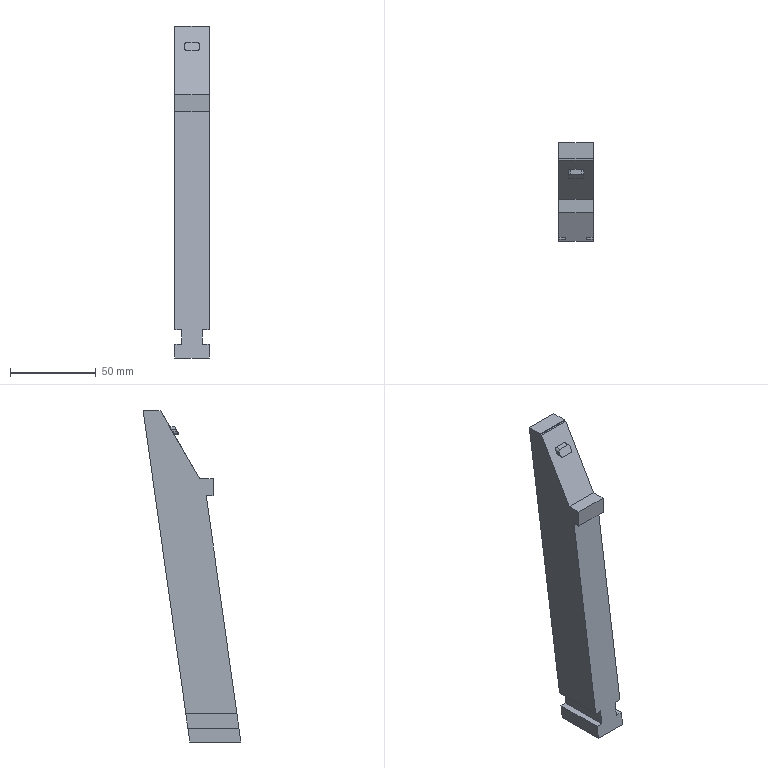Part | NX | features 模具.stp<1>[4] 2 | 1 solid | 29 faces | box 20 x 56.958 x 193.5 mm | volume 105226 mm3 | plane 25 | spline 4
STEP:
#1=CARTESIAN_POINT('',(-63.5,-228.097,-137.));
#2=VERTEX_POINT('',#1);
#3=CARTESIAN_POINT('',(-67.5,-228.097,-137.));
#4=VERTEX_POINT('',#3);
#5=CARTESIAN_POINT('',(38.,-228.097,-137.));
#6=DIRECTION('',(-1.,0.,0.));
#7=VECTOR('',#6,1000.);
#8=LINE('',#5,#7);
#9=EDGE_CURVE('',#2,#4,#8,.T.);
#10=ORIENTED_EDGE('',*,*,#9,.T.);
#11=CARTESIAN_POINT('',(-67.5,-198.334,-137.));
#12=VERTEX_POINT('',#11);
#13=CARTESIAN_POINT('',(-67.5,-264.,-137.));
#14=DIRECTION('',(0.,1.,0.));
#15=VECTOR('',#14,1000.);
#16=LINE('',#13,#15);
#17=EDGE_CURVE('',#4,#12,#16,.T.);
#18=ORIENTED_EDGE('',*,*,#17,.T.);
#19=CARTESIAN_POINT('',(-63.5,-198.334,-137.));
#20=VERTEX_POINT('',#19);
#21=CARTESIAN_POINT('',(38.,-198.334,-137.));
#22=DIRECTION('',(1.,0.,0.));
#23=VECTOR('',#22,1000.);
#24=LINE('',#21,#23);
#25=EDGE_CURVE('',#12,#20,#24,.T.);
#26=ORIENTED_EDGE('',*,*,#25,.T.);
#27=CARTESIAN_POINT('',(-63.5,-264.,-137.));
#28=DIRECTION('',(0.,-1.,0.));
#29=VECTOR('',#28,1000.);
#30=LINE('',#27,#29);
#31=EDGE_CURVE('',#20,#2,#30,.T.);
#32=ORIENTED_EDGE('',*,*,#31,.T.);
#33=EDGE_LOOP('',(#10,#18,#26,#32));
#34=FACE_BOUND('',#33,.T.);
#35=CARTESIAN_POINT('',(-63.5,-264.,-137.));
#36=DIRECTION('',(0.,0.,-1.));
#37=DIRECTION('',(-1.,0.,0.));
#38=AXIS2_PLACEMENT_3D('',#35,#36,#37);
#39=PLANE('',#38);
#40=ADVANCED_FACE('',(#34),#39,.T.);
#41=CARTESIAN_POINT('',(-63.5,-229.292,-145.5));
#42=VERTEX_POINT('',#41);
#43=CARTESIAN_POINT('',(-63.5,-210.249,-10.));
#44=DIRECTION('',(0.,0.1392,0.9903));
#45=VECTOR('',#44,1000.);
#46=LINE('',#43,#45);
#47=EDGE_CURVE('',#42,#2,#46,.T.);
#48=ORIENTED_EDGE('',*,*,#47,.T.);
#49=ORIENTED_EDGE('',*,*,#31,.F.);
#50=CARTESIAN_POINT('',(-63.5,-199.528,-145.5));
#51=VERTEX_POINT('',#50);
#52=CARTESIAN_POINT('',(-63.5,-193.248,-100.81));
#53=DIRECTION('',(0.,-0.1392,-0.9903));
#54=VECTOR('',#53,1000.);
#55=LINE('',#52,#54);
#56=EDGE_CURVE('',#20,#51,#55,.T.);
#57=ORIENTED_EDGE('',*,*,#56,.T.);
#58=CARTESIAN_POINT('',(-63.5,-264.,-145.5));
#59=DIRECTION('',(0.,-1.,0.));
#60=VECTOR('',#59,1000.);
#61=LINE('',#58,#60);
#62=EDGE_CURVE('',#51,#42,#61,.T.);
#63=ORIENTED_EDGE('',*,*,#62,.T.);
#64=EDGE_LOOP('',(#48,#49,#57,#63));
#65=FACE_BOUND('',#64,.T.);
#66=CARTESIAN_POINT('',(-63.5,-264.,-145.5));
#67=DIRECTION('',(-1.,0.,0.));
#68=DIRECTION('',(0.,0.,1.));
#69=AXIS2_PLACEMENT_3D('',#66,#67,#68);
#70=PLANE('',#69);
#71=ADVANCED_FACE('',(#65),#70,.T.);
#72=CARTESIAN_POINT('',(-67.5,-229.292,-145.5));
#73=VERTEX_POINT('',#72);
#74=CARTESIAN_POINT('',(38.,-229.292,-145.5));
#75=DIRECTION('',(1.,0.,0.));
#76=VECTOR('',#75,1000.);
#77=LINE('',#74,#76);
#78=EDGE_CURVE('',#73,#42,#77,.T.);
#79=ORIENTED_EDGE('',*,*,#78,.T.);
#80=ORIENTED_EDGE('',*,*,#62,.F.);
#81=CARTESIAN_POINT('',(-67.5,-199.528,-145.5));
#82=VERTEX_POINT('',#81);
#83=CARTESIAN_POINT('',(38.,-199.528,-145.5));
#84=DIRECTION('',(-1.,0.,0.));
#85=VECTOR('',#84,1000.);
#86=LINE('',#83,#85);
#87=EDGE_CURVE('',#51,#82,#86,.T.);
#88=ORIENTED_EDGE('',*,*,#87,.T.);
#89=CARTESIAN_POINT('',(-67.5,-264.,-145.5));
#90=DIRECTION('',(0.,1.,0.));
#91=VECTOR('',#90,1000.);
#92=LINE('',#89,#91);
#93=EDGE_CURVE('',#73,#82,#92,.T.);
#94=ORIENTED_EDGE('',*,*,#93,.F.);
#95=EDGE_LOOP('',(#79,#80,#88,#94));
#96=FACE_BOUND('',#95,.T.);
#97=CARTESIAN_POINT('',(-67.5,-264.,-145.5));
#98=DIRECTION('',(0.,0.,1.));
#99=DIRECTION('',(1.,0.,0.));
#100=AXIS2_PLACEMENT_3D('',#97,#98,#99);
#101=PLANE('',#100);
#102=ADVANCED_FACE('',(#96),#101,.T.);
#103=CARTESIAN_POINT('',(-47.5,-228.097,-137.));
#104=VERTEX_POINT('',#103);
#105=CARTESIAN_POINT('',(-51.5,-228.097,-137.));
#106=VERTEX_POINT('',#105);
#107=CARTESIAN_POINT('',(38.,-228.097,-137.));
#108=DIRECTION('',(-1.,0.,0.));
#109=VECTOR('',#108,1000.);
#110=LINE('',#107,#109);
#111=EDGE_CURVE('',#104,#106,#110,.T.);
#112=ORIENTED_EDGE('',*,*,#111,.T.);
#113=CARTESIAN_POINT('',(-51.5,-198.334,-137.));
#114=VERTEX_POINT('',#113);
#115=CARTESIAN_POINT('',(-51.5,-264.,-137.));
#116=DIRECTION('',(0.,1.,0.));
#117=VECTOR('',#116,1000.);
#118=LINE('',#115,#117);
#119=EDGE_CURVE('',#106,#114,#118,.T.);
#120=ORIENTED_EDGE('',*,*,#119,.T.);
#121=CARTESIAN_POINT('',(-47.5,-198.334,-137.));
#122=VERTEX_POINT('',#121);
#123=CARTESIAN_POINT('',(38.,-198.334,-137.));
#124=DIRECTION('',(1.,0.,0.));
#125=VECTOR('',#124,1000.);
#126=LINE('',#123,#125);
#127=EDGE_CURVE('',#114,#122,#126,.T.);
#128=ORIENTED_EDGE('',*,*,#127,.T.);
#129=CARTESIAN_POINT('',(-47.5,-264.,-137.));
#130=DIRECTION('',(0.,-1.,0.));
#131=VECTOR('',#130,1000.);
#132=LINE('',#129,#131);
#133=EDGE_CURVE('',#122,#104,#132,.T.);
#134=ORIENTED_EDGE('',*,*,#133,.T.);
#135=EDGE_LOOP('',(#112,#120,#128,#134));
#136=FACE_BOUND('',#135,.T.);
#137=CARTESIAN_POINT('',(-51.5,-264.,-137.));
#138=DIRECTION('',(0.,0.,-1.));
#139=DIRECTION('',(0.,-1.,0.));
#140=AXIS2_PLACEMENT_3D('',#137,#138,#139);
#141=PLANE('',#140);
#142=ADVANCED_FACE('',(#136),#141,.T.);
#143=CARTESIAN_POINT('',(-51.5,-229.292,-145.5));
#144=VERTEX_POINT('',#143);
#145=CARTESIAN_POINT('',(-51.5,-210.249,-10.));
#146=DIRECTION('',(0.,-0.1392,-0.9903));
#147=VECTOR('',#146,1000.);
#148=LINE('',#145,#147);
#149=EDGE_CURVE('',#106,#144,#148,.T.);
#150=ORIENTED_EDGE('',*,*,#149,.T.);
#151=CARTESIAN_POINT('',(-51.5,-199.528,-145.5));
#152=VERTEX_POINT('',#151);
#153=CARTESIAN_POINT('',(-51.5,-264.,-145.5));
#154=DIRECTION('',(0.,1.,0.));
#155=VECTOR('',#154,1000.);
#156=LINE('',#153,#155);
#157=EDGE_CURVE('',#144,#152,#156,.T.);
#158=ORIENTED_EDGE('',*,*,#157,.T.);
#159=CARTESIAN_POINT('',(-51.5,-193.248,-100.81));
#160=DIRECTION('',(0.,0.1392,0.9903));
#161=VECTOR('',#160,1000.);
#162=LINE('',#159,#161);
#163=EDGE_CURVE('',#152,#114,#162,.T.);
#164=ORIENTED_EDGE('',*,*,#163,.T.);
#165=ORIENTED_EDGE('',*,*,#119,.F.);
#166=EDGE_LOOP('',(#150,#158,#164,#165));
#167=FACE_BOUND('',#166,.T.);
#168=CARTESIAN_POINT('',(-51.5,-264.,-145.5));
#169=DIRECTION('',(1.,0.,0.));
#170=DIRECTION('',(0.,0.,-1.));
#171=AXIS2_PLACEMENT_3D('',#168,#169,#170);
#172=PLANE('',#171);
#173=ADVANCED_FACE('',(#167),#172,.T.);
#174=CARTESIAN_POINT('',(-47.5,-229.292,-145.5));
#175=VERTEX_POINT('',#174);
#176=CARTESIAN_POINT('',(38.,-229.292,-145.5));
#177=DIRECTION('',(1.,0.,0.));
#178=VECTOR('',#177,1000.);
#179=LINE('',#176,#178);
#180=EDGE_CURVE('',#144,#175,#179,.T.);
#181=ORIENTED_EDGE('',*,*,#180,.T.);
#182=CARTESIAN_POINT('',(-47.5,-199.528,-145.5));
#183=VERTEX_POINT('',#182);
#184=CARTESIAN_POINT('',(-47.5,-264.,-145.5));
#185=DIRECTION('',(0.,-1.,0.));
#186=VECTOR('',#185,1000.);
#187=LINE('',#184,#186);
#188=EDGE_CURVE('',#183,#175,#187,.T.);
#189=ORIENTED_EDGE('',*,*,#188,.F.);
#190=CARTESIAN_POINT('',(38.,-199.528,-145.5));
#191=DIRECTION('',(-1.,0.,0.));
#192=VECTOR('',#191,1000.);
#193=LINE('',#190,#192);
#194=EDGE_CURVE('',#183,#152,#193,.T.);
#195=ORIENTED_EDGE('',*,*,#194,.T.);
#196=ORIENTED_EDGE('',*,*,#157,.F.);
#197=EDGE_LOOP('',(#181,#189,#195,#196));
#198=FACE_BOUND('',#197,.T.);
#199=CARTESIAN_POINT('',(-47.5,-264.,-145.5));
#200=DIRECTION('',(0.,0.,1.));
#201=DIRECTION('',(1.,0.,0.));
#202=AXIS2_PLACEMENT_3D('',#199,#200,#201);
#203=PLANE('',#202);
#204=ADVANCED_FACE('',(#198),#203,.T.);
#205=CARTESIAN_POINT('',(-60.5,-191.803,30.217));
#206=VERTEX_POINT('',#205);
#207=CARTESIAN_POINT('',(-54.5,-191.803,30.217));
#208=VERTEX_POINT('',#207);
#209=CARTESIAN_POINT('',(0.,-191.803,30.217));
#210=DIRECTION('',(1.,0.,0.));
#211=VECTOR('',#210,1000.);
#212=LINE('',#209,#211);
#213=EDGE_CURVE('',#206,#208,#212,.T.);
#214=ORIENTED_EDGE('',*,*,#213,.F.);
#215=CARTESIAN_POINT('',(-62.,-192.553,28.917));
#216=VERTEX_POINT('',#215);
#217=CARTESIAN_POINT('',(-62.,-192.553,28.917));
#218=CARTESIAN_POINT('',(-62.,-192.455,29.088));
#219=CARTESIAN_POINT('',(-61.961,-192.357,29.258));
#220=CARTESIAN_POINT('',(-61.811,-192.175,29.572));
#221=CARTESIAN_POINT('',(-61.7,-192.092,29.716));
#222=CARTESIAN_POINT('',(-61.422,-191.953,29.956));
#223=CARTESIAN_POINT('',(-61.255,-191.898,30.053));
#224=CARTESIAN_POINT('',(-60.893,-191.823,30.183));
#225=CARTESIAN_POINT('',(-60.696,-191.803,30.217));
#226=CARTESIAN_POINT('',(-60.5,-191.803,30.217));
#227=B_SPLINE_CURVE_WITH_KNOTS('',3,(#217,#218,#219,#220,#221,#222,#223,#224,#225,#226),.UNSPECIFIED.,.F.,.F.,(4,2,2,2,4),(0.,0.25,0.5,0.75,1.),.UNSPECIFIED.);
#228=EDGE_CURVE('',#216,#206,#227,.T.);
#229=ORIENTED_EDGE('',*,*,#228,.F.);
#230=CARTESIAN_POINT('',(-62.,-193.553,27.185));
#231=VERTEX_POINT('',#230);
#232=CARTESIAN_POINT('',(-62.,-197.846,19.75));
#233=DIRECTION('',(0.,-0.5,-0.866));
#234=VECTOR('',#233,1000.);
#235=LINE('',#232,#234);
#236=EDGE_CURVE('',#216,#231,#235,.T.);
#237=ORIENTED_EDGE('',*,*,#236,.T.);
#238=CARTESIAN_POINT('',(-60.5,-194.303,25.886));
#239=VERTEX_POINT('',#238);
#240=CARTESIAN_POINT('',(-60.5,-194.303,25.886));
#241=CARTESIAN_POINT('',(-60.304,-194.303,25.886));
#242=CARTESIAN_POINT('',(-60.107,-194.284,25.92));
#243=CARTESIAN_POINT('',(-59.745,-194.209,26.05));
#244=CARTESIAN_POINT('',(-59.578,-194.153,26.147));
#245=CARTESIAN_POINT('',(-59.3,-194.014,26.387));
#246=CARTESIAN_POINT('',(-59.189,-193.931,26.531));
#247=CARTESIAN_POINT('',(-59.039,-193.749,26.845));
#248=CARTESIAN_POINT('',(-59.,-193.651,27.015));
#249=CARTESIAN_POINT('',(-59.,-193.455,27.355));
#250=CARTESIAN_POINT('',(-59.039,-193.357,27.525));
#251=CARTESIAN_POINT('',(-59.189,-193.175,27.84));
#252=CARTESIAN_POINT('',(-59.3,-193.092,27.984));
#253=CARTESIAN_POINT('',(-59.578,-192.953,28.224));
#254=CARTESIAN_POINT('',(-59.745,-192.898,28.321));
#255=CARTESIAN_POINT('',(-60.107,-192.823,28.451));
#256=CARTESIAN_POINT('',(-60.304,-192.803,28.484));
#257=CARTESIAN_POINT('',(-60.696,-192.803,28.484));
#258=CARTESIAN_POINT('',(-60.893,-192.823,28.451));
#259=CARTESIAN_POINT('',(-61.255,-192.898,28.321));
#260=CARTESIAN_POINT('',(-61.422,-192.953,28.224));
#261=CARTESIAN_POINT('',(-61.7,-193.092,27.984));
#262=CARTESIAN_POINT('',(-61.811,-193.175,27.84));
#263=CARTESIAN_POINT('',(-61.961,-193.357,27.525));
#264=CARTESIAN_POINT('',(-62.,-193.455,27.355));
#265=CARTESIAN_POINT('',(-62.,-193.651,27.015));
#266=CARTESIAN_POINT('',(-61.961,-193.749,26.845));
#267=CARTESIAN_POINT('',(-61.811,-193.931,26.531));
#268=CARTESIAN_POINT('',(-61.7,-194.014,26.387));
#269=CARTESIAN_POINT('',(-61.422,-194.153,26.147));
#270=CARTESIAN_POINT('',(-61.255,-194.209,26.05));
#271=CARTESIAN_POINT('',(-60.893,-194.284,25.92));
#272=CARTESIAN_POINT('',(-60.696,-194.303,25.886));
#273=CARTESIAN_POINT('',(-60.5,-194.303,25.886));
#274=B_SPLINE_CURVE_WITH_KNOTS('',3,(#240,#241,#242,#243,#244,#245,#246,#247,#248,#249,#250,#251,#252,#253,#254,#255,#256,#257,#258,#259,#260,#261,#262,#263,#264,#265,#266,#267,#268,#269,#270,#271,#272,#273),.UNSPECIFIED.,.T.,.F.,(1,3,2,2,2,2,2,2,2,2,2,2,2,2,2,2,2,3,1),(-0.0625,0.,0.0625,0.125,0.1875,0.25,0.3125,0.375,0.4375,0.5,0.5625,0.625,0.6875,0.75,0.8125,0.875,0.9375,1.,1.062),.UNSPECIFIED.);
#275=EDGE_CURVE('',#231,#239,#274,.T.);
#276=ORIENTED_EDGE('',*,*,#275,.T.);
#277=CARTESIAN_POINT('',(-54.5,-194.303,25.886));
#278=VERTEX_POINT('',#277);
#279=CARTESIAN_POINT('',(0.,-194.303,25.886));
#280=DIRECTION('',(1.,0.,0.));
#281=VECTOR('',#280,1000.);
#282=LINE('',#279,#281);
#283=EDGE_CURVE('',#239,#278,#282,.T.);
#284=ORIENTED_EDGE('',*,*,#283,.T.);
#285=CARTESIAN_POINT('',(-53.,-193.553,27.185));
#286=VERTEX_POINT('',#285);
#287=CARTESIAN_POINT('',(-54.5,-194.303,25.886));
#288=CARTESIAN_POINT('',(-54.696,-194.303,25.886));
#289=CARTESIAN_POINT('',(-54.893,-194.284,25.92));
#290=CARTESIAN_POINT('',(-55.255,-194.209,26.05));
#291=CARTESIAN_POINT('',(-55.422,-194.153,26.147));
#292=CARTESIAN_POINT('',(-55.7,-194.014,26.387));
#293=CARTESIAN_POINT('',(-55.811,-193.931,26.531));
#294=CARTESIAN_POINT('',(-55.961,-193.749,26.845));
#295=CARTESIAN_POINT('',(-56.,-193.651,27.015));
#296=CARTESIAN_POINT('',(-56.,-193.455,27.355));
#297=CARTESIAN_POINT('',(-55.961,-193.357,27.525));
#298=CARTESIAN_POINT('',(-55.811,-193.175,27.84));
#299=CARTESIAN_POINT('',(-55.7,-193.092,27.984));
#300=CARTESIAN_POINT('',(-55.422,-192.953,28.224));
#301=CARTESIAN_POINT('',(-55.255,-192.898,28.321));
#302=CARTESIAN_POINT('',(-54.893,-192.823,28.451));
#303=CARTESIAN_POINT('',(-54.696,-192.803,28.484));
#304=CARTESIAN_POINT('',(-54.304,-192.803,28.484));
#305=CARTESIAN_POINT('',(-54.107,-192.823,28.451));
#306=CARTESIAN_POINT('',(-53.745,-192.898,28.321));
#307=CARTESIAN_POINT('',(-53.578,-192.953,28.224));
#308=CARTESIAN_POINT('',(-53.3,-193.092,27.984));
#309=CARTESIAN_POINT('',(-53.189,-193.175,27.84));
#310=CARTESIAN_POINT('',(-53.039,-193.357,27.525));
#311=CARTESIAN_POINT('',(-53.,-193.455,27.355));
#312=CARTESIAN_POINT('',(-53.,-193.651,27.015));
#313=CARTESIAN_POINT('',(-53.039,-193.749,26.845));
#314=CARTESIAN_POINT('',(-53.189,-193.931,26.531));
#315=CARTESIAN_POINT('',(-53.3,-194.014,26.387));
#316=CARTESIAN_POINT('',(-53.578,-194.153,26.147));
#317=CARTESIAN_POINT('',(-53.745,-194.209,26.05));
#318=CARTESIAN_POINT('',(-54.107,-194.284,25.92));
#319=CARTESIAN_POINT('',(-54.304,-194.303,25.886));
#320=CARTESIAN_POINT('',(-54.5,-194.303,25.886));
#321=B_SPLINE_CURVE_WITH_KNOTS('',3,(#287,#288,#289,#290,#291,#292,#293,#294,#295,#296,#297,#298,#299,#300,#301,#302,#303,#304,#305,#306,#307,#308,#309,#310,#311,#312,#313,#314,#315,#316,#317,#318,#319,#320),.UNSPECIFIED.,.T.,.F.,(1,3,2,2,2,2,2,2,2,2,2,2,2,2,2,2,2,3,1),(-0.0625,0.,0.0625,0.125,0.1875,0.25,0.3125,0.375,0.4375,0.5,0.5625,0.625,0.6875,0.75,0.8125,0.875,0.9375,1.,1.062),.UNSPECIFIED.);
#322=EDGE_CURVE('',#286,#278,#321,.T.);
#323=ORIENTED_EDGE('',*,*,#322,.F.);
#324=CARTESIAN_POINT('',(-53.,-192.553,28.917));
#325=VERTEX_POINT('',#324);
#326=CARTESIAN_POINT('',(-53.,-197.846,19.75));
#327=DIRECTION('',(0.,-0.5,-0.866));
#328=VECTOR('',#327,1000.);
#329=LINE('',#326,#328);
#330=EDGE_CURVE('',#325,#286,#329,.T.);
#331=ORIENTED_EDGE('',*,*,#330,.F.);
#332=CARTESIAN_POINT('',(-54.5,-193.303,27.618));
#333=CARTESIAN_POINT('',(-54.696,-193.303,27.618));
#334=CARTESIAN_POINT('',(-54.893,-193.284,27.652));
#335=CARTESIAN_POINT('',(-55.255,-193.209,27.782));
#336=CARTESIAN_POINT('',(-55.422,-193.153,27.879));
#337=CARTESIAN_POINT('',(-55.7,-193.014,28.119));
#338=CARTESIAN_POINT('',(-55.811,-192.931,28.263));
#339=CARTESIAN_POINT('',(-55.961,-192.749,28.577));
#340=CARTESIAN_POINT('',(-56.,-192.651,28.747));
#341=CARTESIAN_POINT('',(-56.,-192.455,29.088));
#342=CARTESIAN_POINT('',(-55.961,-192.357,29.258));
#343=CARTESIAN_POINT('',(-55.811,-192.175,29.572));
#344=CARTESIAN_POINT('',(-55.7,-192.092,29.716));
#345=CARTESIAN_POINT('',(-55.422,-191.953,29.956));
#346=CARTESIAN_POINT('',(-55.255,-191.898,30.053));
#347=CARTESIAN_POINT('',(-54.893,-191.823,30.183));
#348=CARTESIAN_POINT('',(-54.696,-191.803,30.217));
#349=CARTESIAN_POINT('',(-54.304,-191.803,30.217));
#350=CARTESIAN_POINT('',(-54.107,-191.823,30.183));
#351=CARTESIAN_POINT('',(-53.745,-191.898,30.053));
#352=CARTESIAN_POINT('',(-53.578,-191.953,29.956));
#353=CARTESIAN_POINT('',(-53.3,-192.092,29.716));
#354=CARTESIAN_POINT('',(-53.189,-192.175,29.572));
#355=CARTESIAN_POINT('',(-53.039,-192.357,29.258));
#356=CARTESIAN_POINT('',(-53.,-192.455,29.088));
#357=CARTESIAN_POINT('',(-53.,-192.651,28.747));
#358=CARTESIAN_POINT('',(-53.039,-192.749,28.577));
#359=CARTESIAN_POINT('',(-53.189,-192.931,28.263));
#360=CARTESIAN_POINT('',(-53.3,-193.014,28.119));
#361=CARTESIAN_POINT('',(-53.578,-193.153,27.879));
#362=CARTESIAN_POINT('',(-53.745,-193.209,27.782));
#363=CARTESIAN_POINT('',(-54.107,-193.284,27.652));
#364=CARTESIAN_POINT('',(-54.304,-193.303,27.618));
#365=CARTESIAN_POINT('',(-54.5,-193.303,27.618));
#366=B_SPLINE_CURVE_WITH_KNOTS('',3,(#332,#333,#334,#335,#336,#337,#338,#339,#340,#341,#342,#343,#344,#345,#346,#347,#348,#349,#350,#351,#352,#353,#354,#355,#356,#357,#358,#359,#360,#361,#362,#363,#364,#365),.UNSPECIFIED.,.T.,.F.,(1,3,2,2,2,2,2,2,2,2,2,2,2,2,2,2,2,3,1),(-0.0625,0.,0.0625,0.125,0.1875,0.25,0.3125,0.375,0.4375,0.5,0.5625,0.625,0.6875,0.75,0.8125,0.875,0.9375,1.,1.062),.UNSPECIFIED.);
#367=EDGE_CURVE('',#208,#325,#366,.T.);
#368=ORIENTED_EDGE('',*,*,#367,.F.);
#369=EDGE_LOOP('',(#214,#229,#237,#276,#284,#323,#331,#368));
#370=FACE_BOUND('',#369,.T.);
#371=CARTESIAN_POINT('',(-337.196,-186.443,39.5));
#372=DIRECTION('',(0.,-0.866,0.5));
#373=DIRECTION('',(-1.,0.,0.));
#374=AXIS2_PLACEMENT_3D('',#371,#372,#373);
#375=PLANE('',#374);
#376=ADVANCED_FACE('',(#370),#375,.T.);
#377=CARTESIAN_POINT('',(-60.5,-188.916,30.217));
#378=VERTEX_POINT('',#377);
#379=CARTESIAN_POINT('',(-62.,-189.666,28.917));
#380=VERTEX_POINT('',#379);
#381=CARTESIAN_POINT('',(-60.5,-188.916,30.217));
#382=CARTESIAN_POINT('',(-60.696,-188.916,30.217));
#383=CARTESIAN_POINT('',(-60.893,-188.936,30.183));
#384=CARTESIAN_POINT('',(-61.255,-189.011,30.053));
#385=CARTESIAN_POINT('',(-61.422,-189.067,29.956));
#386=CARTESIAN_POINT('',(-61.7,-189.206,29.716));
#387=CARTESIAN_POINT('',(-61.811,-189.289,29.572));
#388=CARTESIAN_POINT('',(-61.961,-189.47,29.258));
#389=CARTESIAN_POINT('',(-62.,-189.568,29.088));
#390=CARTESIAN_POINT('',(-62.,-189.666,28.917));
#391=B_SPLINE_CURVE_WITH_KNOTS('',3,(#381,#382,#383,#384,#385,#386,#387,#388,#389,#390),.UNSPECIFIED.,.F.,.F.,(4,2,2,2,4),(0.,0.25,0.5,0.75,1.),.UNSPECIFIED.);
#392=EDGE_CURVE('',#378,#380,#391,.T.);
#393=ORIENTED_EDGE('',*,*,#392,.T.);
#394=CARTESIAN_POINT('',(-62.,-192.553,28.917));
#395=DIRECTION('',(0.,1.,0.));
#396=VECTOR('',#395,1000.);
#397=LINE('',#394,#396);
#398=EDGE_CURVE('',#216,#380,#397,.T.);
#399=ORIENTED_EDGE('',*,*,#398,.F.);
#400=ORIENTED_EDGE('',*,*,#228,.T.);
#401=CARTESIAN_POINT('',(-60.5,-191.803,30.217));
#402=DIRECTION('',(0.,1.,0.));
#403=VECTOR('',#402,1000.);
#404=LINE('',#401,#403);
#405=EDGE_CURVE('',#206,#378,#404,.T.);
#406=ORIENTED_EDGE('',*,*,#405,.T.);
#407=EDGE_LOOP('',(#393,#399,#400,#406));
#408=FACE_BOUND('',#407,.T.);
#409=CARTESIAN_POINT('',(-60.5,-191.803,30.217));
#410=CARTESIAN_POINT('',(-60.696,-191.803,30.217));
#411=CARTESIAN_POINT('',(-60.893,-191.823,30.183));
#412=CARTESIAN_POINT('',(-61.255,-191.898,30.053));
#413=CARTESIAN_POINT('',(-61.422,-191.953,29.956));
#414=CARTESIAN_POINT('',(-61.7,-192.092,29.716));
#415=CARTESIAN_POINT('',(-61.811,-192.175,29.572));
#416=CARTESIAN_POINT('',(-61.961,-192.357,29.258));
#417=CARTESIAN_POINT('',(-62.,-192.455,29.088));
#418=CARTESIAN_POINT('',(-62.,-192.553,28.917));
#419=CARTESIAN_POINT('',(-60.5,-188.916,30.217));
#420=CARTESIAN_POINT('',(-60.696,-188.916,30.217));
#421=CARTESIAN_POINT('',(-60.893,-188.936,30.183));
#422=CARTESIAN_POINT('',(-61.255,-189.011,30.053));
#423=CARTESIAN_POINT('',(-61.422,-189.067,29.956));
#424=CARTESIAN_POINT('',(-61.7,-189.206,29.716));
#425=CARTESIAN_POINT('',(-61.811,-189.289,29.572));
#426=CARTESIAN_POINT('',(-61.961,-189.47,29.258));
#427=CARTESIAN_POINT('',(-62.,-189.568,29.088));
#428=CARTESIAN_POINT('',(-62.,-189.666,28.917));
#429=B_SPLINE_SURFACE_WITH_KNOTS('',1,3,((#409,#410,#411,#412,#413,#414,#415,#416,#417,#418),(#419,#420,#421,#422,#423,#424,#425,#426,#427,#428)),.SURF_OF_LINEAR_EXTRUSION.,.F.,.F.,.F.,(2,2),(4,2,2,2,4),(0.1699,0.7147),(0.5,0.5625,0.625,0.6875,0.75),.UNSPECIFIED.);
#430=ADVANCED_FACE('',(#408),#429,.T.);
#431=ORIENTED_EDGE('',*,*,#398,.T.);
#432=CARTESIAN_POINT('',(-62.,-190.666,27.185));
#433=VERTEX_POINT('',#432);
#434=CARTESIAN_POINT('',(-62.,-182.835,40.75));
#435=DIRECTION('',(0.,0.5,0.866));
#436=VECTOR('',#435,1000.);
#437=LINE('',#434,#436);
#438=EDGE_CURVE('',#433,#380,#437,.T.);
#439=ORIENTED_EDGE('',*,*,#438,.F.);
#440=CARTESIAN_POINT('',(-62.,-193.553,27.185));
#441=DIRECTION('',(0.,1.,0.));
#442=VECTOR('',#441,1000.);
#443=LINE('',#440,#442);
#444=EDGE_CURVE('',#231,#433,#443,.T.);
#445=ORIENTED_EDGE('',*,*,#444,.F.);
#446=ORIENTED_EDGE('',*,*,#236,.F.);
#447=EDGE_LOOP('',(#431,#439,#445,#446));
#448=FACE_BOUND('',#447,.T.);
#449=CARTESIAN_POINT('',(-62.,-197.846,19.75));
#450=DIRECTION('',(1.,0.,0.));
#451=DIRECTION('',(0.,0.,-1.));
#452=AXIS2_PLACEMENT_3D('',#449,#450,#451);
#453=PLANE('',#452);
#454=ADVANCED_FACE('',(#448),#453,.F.);
#455=ORIENTED_EDGE('',*,*,#444,.T.);
#456=CARTESIAN_POINT('',(-60.5,-191.416,25.886));
#457=VERTEX_POINT('',#456);
#458=CARTESIAN_POINT('',(-60.5,-191.416,25.886));
#459=CARTESIAN_POINT('',(-60.696,-191.416,25.886));
#460=CARTESIAN_POINT('',(-60.893,-191.397,25.92));
#461=CARTESIAN_POINT('',(-61.255,-191.322,26.05));
#462=CARTESIAN_POINT('',(-61.422,-191.266,26.147));
#463=CARTESIAN_POINT('',(-61.7,-191.127,26.387));
#464=CARTESIAN_POINT('',(-61.811,-191.044,26.531));
#465=CARTESIAN_POINT('',(-61.961,-190.863,26.845));
#466=CARTESIAN_POINT('',(-62.,-190.765,27.015));
#467=CARTESIAN_POINT('',(-62.,-190.666,27.185));
#468=B_SPLINE_CURVE_WITH_KNOTS('',3,(#458,#459,#460,#461,#462,#463,#464,#465,#466,#467),.UNSPECIFIED.,.F.,.F.,(4,2,2,2,4),(0.,0.25,0.5,0.75,1.),.UNSPECIFIED.);
#469=EDGE_CURVE('',#457,#433,#468,.T.);
#470=ORIENTED_EDGE('',*,*,#469,.F.);
#471=CARTESIAN_POINT('',(-60.5,-194.303,25.886));
#472=DIRECTION('',(0.,1.,0.));
#473=VECTOR('',#472,1000.);
#474=LINE('',#471,#473);
#475=EDGE_CURVE('',#239,#457,#474,.T.);
#476=ORIENTED_EDGE('',*,*,#475,.F.);
#477=ORIENTED_EDGE('',*,*,#275,.F.);
#478=EDGE_LOOP('',(#455,#470,#476,#477));
#479=FACE_BOUND('',#478,.T.);
#480=CARTESIAN_POINT('',(-62.,-193.553,27.185));
#481=CARTESIAN_POINT('',(-62.,-193.651,27.015));
#482=CARTESIAN_POINT('',(-61.961,-193.749,26.845));
#483=CARTESIAN_POINT('',(-61.811,-193.931,26.531));
#484=CARTESIAN_POINT('',(-61.7,-194.014,26.387));
#485=CARTESIAN_POINT('',(-61.422,-194.153,26.147));
#486=CARTESIAN_POINT('',(-61.255,-194.209,26.05));
#487=CARTESIAN_POINT('',(-60.893,-194.284,25.92));
#488=CARTESIAN_POINT('',(-60.696,-194.303,25.886));
#489=CARTESIAN_POINT('',(-60.5,-194.303,25.886));
#490=CARTESIAN_POINT('',(-62.,-190.666,27.185));
#491=CARTESIAN_POINT('',(-62.,-190.765,27.015));
#492=CARTESIAN_POINT('',(-61.961,-190.863,26.845));
#493=CARTESIAN_POINT('',(-61.811,-191.044,26.531));
#494=CARTESIAN_POINT('',(-61.7,-191.127,26.387));
#495=CARTESIAN_POINT('',(-61.422,-191.266,26.147));
#496=CARTESIAN_POINT('',(-61.255,-191.322,26.05));
#497=CARTESIAN_POINT('',(-60.893,-191.397,25.92));
#498=CARTESIAN_POINT('',(-60.696,-191.416,25.886));
#499=CARTESIAN_POINT('',(-60.5,-191.416,25.886));
#500=B_SPLINE_SURFACE_WITH_KNOTS('',1,3,((#480,#481,#482,#483,#484,#485,#486,#487,#488,#489),(#490,#491,#492,#493,#494,#495,#496,#497,#498,#499)),.SURF_OF_LINEAR_EXTRUSION.,.F.,.F.,.F.,(2,2),(4,2,2,2,4),(0.3397,0.8846),(0.75,0.8125,0.875,0.9375,1.),.UNSPECIFIED.);
#501=ADVANCED_FACE('',(#479),#500,.T.);
#502=ORIENTED_EDGE('',*,*,#475,.T.);
#503=CARTESIAN_POINT('',(-54.5,-191.416,25.886));
#504=VERTEX_POINT('',#503);
#505=CARTESIAN_POINT('',(-89.,-191.416,25.886));
#506=DIRECTION('',(-1.,0.,0.));
#507=VECTOR('',#506,1000.);
#508=LINE('',#505,#507);
#509=EDGE_CURVE('',#504,#457,#508,.T.);
#510=ORIENTED_EDGE('',*,*,#509,.F.);
#511=CARTESIAN_POINT('',(-54.5,-194.303,25.886));
#512=DIRECTION('',(0.,1.,0.));
#513=VECTOR('',#512,1000.);
#514=LINE('',#511,#513);
#515=EDGE_CURVE('',#278,#504,#514,.T.);
#516=ORIENTED_EDGE('',*,*,#515,.F.);
#517=ORIENTED_EDGE('',*,*,#283,.F.);
#518=EDGE_LOOP('',(#502,#510,#516,#517));
#519=FACE_BOUND('',#518,.T.);
#520=CARTESIAN_POINT('',(0.,-194.303,25.886));
#521=DIRECTION('',(0.,0.,1.));
#522=DIRECTION('',(1.,0.,0.));
#523=AXIS2_PLACEMENT_3D('',#520,#521,#522);
#524=PLANE('',#523);
#525=ADVANCED_FACE('',(#519),#524,.F.);
#526=CARTESIAN_POINT('',(-53.,-190.666,27.185));
#527=VERTEX_POINT('',#526);
#528=CARTESIAN_POINT('',(-54.5,-191.416,25.886));
#529=CARTESIAN_POINT('',(-54.304,-191.416,25.886));
#530=CARTESIAN_POINT('',(-54.107,-191.397,25.92));
#531=CARTESIAN_POINT('',(-53.745,-191.322,26.05));
#532=CARTESIAN_POINT('',(-53.578,-191.266,26.147));
#533=CARTESIAN_POINT('',(-53.3,-191.127,26.387));
#534=CARTESIAN_POINT('',(-53.189,-191.044,26.531));
#535=CARTESIAN_POINT('',(-53.039,-190.863,26.845));
#536=CARTESIAN_POINT('',(-53.,-190.765,27.015));
#537=CARTESIAN_POINT('',(-53.,-190.666,27.185));
#538=B_SPLINE_CURVE_WITH_KNOTS('',3,(#528,#529,#530,#531,#532,#533,#534,#535,#536,#537),.UNSPECIFIED.,.F.,.F.,(4,2,2,2,4),(0.,0.25,0.5,0.75,1.),.UNSPECIFIED.);
#539=EDGE_CURVE('',#504,#527,#538,.T.);
#540=ORIENTED_EDGE('',*,*,#539,.T.);
#541=CARTESIAN_POINT('',(-53.,-193.553,27.185));
#542=DIRECTION('',(0.,1.,0.));
#543=VECTOR('',#542,1000.);
#544=LINE('',#541,#543);
#545=EDGE_CURVE('',#286,#527,#544,.T.);
#546=ORIENTED_EDGE('',*,*,#545,.F.);
#547=ORIENTED_EDGE('',*,*,#322,.T.);
#548=ORIENTED_EDGE('',*,*,#515,.T.);
#549=EDGE_LOOP('',(#540,#546,#547,#548));
#550=FACE_BOUND('',#549,.T.);
#551=CARTESIAN_POINT('',(-54.5,-194.303,25.886));
#552=CARTESIAN_POINT('',(-54.304,-194.303,25.886));
#553=CARTESIAN_POINT('',(-54.107,-194.284,25.92));
#554=CARTESIAN_POINT('',(-53.745,-194.209,26.05));
#555=CARTESIAN_POINT('',(-53.578,-194.153,26.147));
#556=CARTESIAN_POINT('',(-53.3,-194.014,26.387));
#557=CARTESIAN_POINT('',(-53.189,-193.931,26.531));
#558=CARTESIAN_POINT('',(-53.039,-193.749,26.845));
#559=CARTESIAN_POINT('',(-53.,-193.651,27.015));
#560=CARTESIAN_POINT('',(-53.,-193.553,27.185));
#561=CARTESIAN_POINT('',(-54.5,-191.416,25.886));
#562=CARTESIAN_POINT('',(-54.304,-191.416,25.886));
#563=CARTESIAN_POINT('',(-54.107,-191.397,25.92));
#564=CARTESIAN_POINT('',(-53.745,-191.322,26.05));
#565=CARTESIAN_POINT('',(-53.578,-191.266,26.147));
#566=CARTESIAN_POINT('',(-53.3,-191.127,26.387));
#567=CARTESIAN_POINT('',(-53.189,-191.044,26.531));
#568=CARTESIAN_POINT('',(-53.039,-190.863,26.845));
#569=CARTESIAN_POINT('',(-53.,-190.765,27.015));
#570=CARTESIAN_POINT('',(-53.,-190.666,27.185));
#571=B_SPLINE_SURFACE_WITH_KNOTS('',1,3,((#551,#552,#553,#554,#555,#556,#557,#558,#559,#560),(#561,#562,#563,#564,#565,#566,#567,#568,#569,#570)),.SURF_OF_LINEAR_EXTRUSION.,.F.,.F.,.F.,(2,2),(4,2,2,2,4),(0.3397,0.8846),(0.,0.0625,0.125,0.1875,0.25),.UNSPECIFIED.);
#572=ADVANCED_FACE('',(#550),#571,.T.);
#573=CARTESIAN_POINT('',(-53.,-189.666,28.917));
#574=VERTEX_POINT('',#573);
#575=CARTESIAN_POINT('',(-53.,-182.835,40.75));
#576=DIRECTION('',(0.,0.5,0.866));
#577=VECTOR('',#576,1000.);
#578=LINE('',#575,#577);
#579=EDGE_CURVE('',#527,#574,#578,.T.);
#580=ORIENTED_EDGE('',*,*,#579,.T.);
#581=CARTESIAN_POINT('',(-53.,-192.553,28.917));
#582=DIRECTION('',(0.,1.,0.));
#583=VECTOR('',#582,1000.);
#584=LINE('',#581,#583);
#585=EDGE_CURVE('',#325,#574,#584,.T.);
#586=ORIENTED_EDGE('',*,*,#585,.F.);
#587=ORIENTED_EDGE('',*,*,#330,.T.);
#588=ORIENTED_EDGE('',*,*,#545,.T.);
#589=EDGE_LOOP('',(#580,#586,#587,#588));
#590=FACE_BOUND('',#589,.T.);
#591=CARTESIAN_POINT('',(-53.,-197.846,19.75));
#592=DIRECTION('',(-1.,0.,0.));
#593=DIRECTION('',(0.,1.,0.));
#594=AXIS2_PLACEMENT_3D('',#591,#592,#593);
#595=PLANE('',#594);
#596=ADVANCED_FACE('',(#590),#595,.F.);
#597=CARTESIAN_POINT('',(-54.5,-188.916,30.217));
#598=VERTEX_POINT('',#597);
#599=CARTESIAN_POINT('',(-53.,-189.666,28.917));
#600=CARTESIAN_POINT('',(-53.,-189.568,29.088));
#601=CARTESIAN_POINT('',(-53.039,-189.47,29.258));
#602=CARTESIAN_POINT('',(-53.189,-189.289,29.572));
#603=CARTESIAN_POINT('',(-53.3,-189.206,29.716));
#604=CARTESIAN_POINT('',(-53.578,-189.067,29.956));
#605=CARTESIAN_POINT('',(-53.745,-189.011,30.053));
#606=CARTESIAN_POINT('',(-54.107,-188.936,30.183));
#607=CARTESIAN_POINT('',(-54.304,-188.916,30.217));
#608=CARTESIAN_POINT('',(-54.5,-188.916,30.217));
#609=B_SPLINE_CURVE_WITH_KNOTS('',3,(#599,#600,#601,#602,#603,#604,#605,#606,#607,#608),.UNSPECIFIED.,.F.,.F.,(4,2,2,2,4),(0.,0.25,0.5,0.75,1.),.UNSPECIFIED.);
#610=EDGE_CURVE('',#574,#598,#609,.T.);
#611=ORIENTED_EDGE('',*,*,#610,.T.);
#612=CARTESIAN_POINT('',(-54.5,-191.803,30.217));
#613=DIRECTION('',(0.,1.,0.));
#614=VECTOR('',#613,1000.);
#615=LINE('',#612,#614);
#616=EDGE_CURVE('',#208,#598,#615,.T.);
#617=ORIENTED_EDGE('',*,*,#616,.F.);
#618=ORIENTED_EDGE('',*,*,#367,.T.);
#619=ORIENTED_EDGE('',*,*,#585,.T.);
#620=EDGE_LOOP('',(#611,#617,#618,#619));
#621=FACE_BOUND('',#620,.T.);
#622=CARTESIAN_POINT('',(-53.,-192.553,28.917));
#623=CARTESIAN_POINT('',(-53.,-192.455,29.088));
#624=CARTESIAN_POINT('',(-53.039,-192.357,29.258));
#625=CARTESIAN_POINT('',(-53.189,-192.175,29.572));
#626=CARTESIAN_POINT('',(-53.3,-192.092,29.716));
#627=CARTESIAN_POINT('',(-53.578,-191.953,29.956));
#628=CARTESIAN_POINT('',(-53.745,-191.898,30.053));
#629=CARTESIAN_POINT('',(-54.107,-191.823,30.183));
#630=CARTESIAN_POINT('',(-54.304,-191.803,30.217));
#631=CARTESIAN_POINT('',(-54.5,-191.803,30.217));
#632=CARTESIAN_POINT('',(-53.,-189.666,28.917));
#633=CARTESIAN_POINT('',(-53.,-189.568,29.088));
#634=CARTESIAN_POINT('',(-53.039,-189.47,29.258));
#635=CARTESIAN_POINT('',(-53.189,-189.289,29.572));
#636=CARTESIAN_POINT('',(-53.3,-189.206,29.716));
#637=CARTESIAN_POINT('',(-53.578,-189.067,29.956));
#638=CARTESIAN_POINT('',(-53.745,-189.011,30.053));
#639=CARTESIAN_POINT('',(-54.107,-188.936,30.183));
#640=CARTESIAN_POINT('',(-54.304,-188.916,30.217));
#641=CARTESIAN_POINT('',(-54.5,-188.916,30.217));
#642=B_SPLINE_SURFACE_WITH_KNOTS('',1,3,((#622,#623,#624,#625,#626,#627,#628,#629,#630,#631),(#632,#633,#634,#635,#636,#637,#638,#639,#640,#641)),.SURF_OF_LINEAR_EXTRUSION.,.F.,.F.,.F.,(2,2),(4,2,2,2,4),(0.1699,0.7147),(0.25,0.3125,0.375,0.4375,0.5),.UNSPECIFIED.);
#643=ADVANCED_FACE('',(#621),#642,.T.);
#644=CARTESIAN_POINT('',(-89.,-188.916,30.217));
#645=DIRECTION('',(-1.,0.,0.));
#646=VECTOR('',#645,1000.);
#647=LINE('',#644,#646);
#648=EDGE_CURVE('',#598,#378,#647,.T.);
#649=ORIENTED_EDGE('',*,*,#648,.T.);
#650=ORIENTED_EDGE('',*,*,#405,.F.);
#651=ORIENTED_EDGE('',*,*,#213,.T.);
#652=ORIENTED_EDGE('',*,*,#616,.T.);
#653=EDGE_LOOP('',(#649,#650,#651,#652));
#654=FACE_BOUND('',#653,.T.);
#655=CARTESIAN_POINT('',(0.,-191.803,30.217));
#656=DIRECTION('',(0.,0.,-1.));
#657=DIRECTION('',(-1.,0.,0.));
#658=AXIS2_PLACEMENT_3D('',#655,#656,#657);
#659=PLANE('',#658);
#660=ADVANCED_FACE('',(#654),#659,.F.);
#661=CARTESIAN_POINT('',(-47.5,-182.5,40.));
#662=VERTEX_POINT('',#661);
#663=CARTESIAN_POINT('',(-47.5,-173.458,40.));
#664=VERTEX_POINT('',#663);
#665=CARTESIAN_POINT('',(-47.5,-197.846,40.));
#666=DIRECTION('',(0.,1.,0.));
#667=VECTOR('',#666,1000.);
#668=LINE('',#665,#667);
#669=EDGE_CURVE('',#662,#664,#668,.T.);
#670=ORIENTED_EDGE('',*,*,#669,.T.);
#671=CARTESIAN_POINT('',(-67.5,-173.458,40.));
#672=VERTEX_POINT('',#671);
#673=CARTESIAN_POINT('',(38.,-173.458,40.));
#674=DIRECTION('',(1.,0.,0.));
#675=VECTOR('',#674,1000.);
#676=LINE('',#673,#675);
#677=EDGE_CURVE('',#672,#664,#676,.T.);
#678=ORIENTED_EDGE('',*,*,#677,.F.);
#679=CARTESIAN_POINT('',(-67.5,-182.5,40.));
#680=VERTEX_POINT('',#679);
#681=CARTESIAN_POINT('',(-67.5,-197.846,40.));
#682=DIRECTION('',(0.,1.,0.));
#683=VECTOR('',#682,1000.);
#684=LINE('',#681,#683);
#685=EDGE_CURVE('',#680,#672,#684,.T.);
#686=ORIENTED_EDGE('',*,*,#685,.F.);
#687=CARTESIAN_POINT('',(-89.,-182.5,40.));
#688=DIRECTION('',(1.,0.,0.));
#689=VECTOR('',#688,1000.);
#690=LINE('',#687,#689);
#691=EDGE_CURVE('',#680,#662,#690,.T.);
#692=ORIENTED_EDGE('',*,*,#691,.T.);
#693=EDGE_LOOP('',(#670,#678,#686,#692));
#694=FACE_BOUND('',#693,.T.);
#695=CARTESIAN_POINT('',(0.,0.,40.));
#696=DIRECTION('',(0.,0.,-1.));
#697=DIRECTION('',(0.,-1.,0.));
#698=AXIS2_PLACEMENT_3D('',#695,#696,#697);
#699=PLANE('',#698);
#700=ADVANCED_FACE('',(#694),#699,.F.);
#701=ORIENTED_EDGE('',*,*,#648,.F.);
#702=ORIENTED_EDGE('',*,*,#610,.F.);
#703=ORIENTED_EDGE('',*,*,#579,.F.);
#704=ORIENTED_EDGE('',*,*,#539,.F.);
#705=ORIENTED_EDGE('',*,*,#509,.T.);
#706=ORIENTED_EDGE('',*,*,#469,.T.);
#707=ORIENTED_EDGE('',*,*,#438,.T.);
#708=ORIENTED_EDGE('',*,*,#392,.F.);
#709=EDGE_LOOP('',(#701,#702,#703,#704,#705,#706,#707,#708));
#710=FACE_BOUND('',#709,.T.);
#711=CARTESIAN_POINT('',(-47.5,-206.362,0.));
#712=VERTEX_POINT('',#711);
#713=CARTESIAN_POINT('',(-47.5,-183.557,39.5));
#714=VERTEX_POINT('',#713);
#715=CARTESIAN_POINT('',(-47.5,-195.681,18.5));
#716=DIRECTION('',(0.,0.5,0.866));
#717=VECTOR('',#716,1000.);
#718=LINE('',#715,#717);
#719=EDGE_CURVE('',#712,#714,#718,.T.);
#720=ORIENTED_EDGE('',*,*,#719,.T.);
#721=CARTESIAN_POINT('',(-67.5,-183.557,39.5));
#722=VERTEX_POINT('',#721);
#723=CARTESIAN_POINT('',(0.,-183.557,39.5));
#724=DIRECTION('',(-1.,0.,0.));
#725=VECTOR('',#724,1000.);
#726=LINE('',#723,#725);
#727=EDGE_CURVE('',#714,#722,#726,.T.);
#728=ORIENTED_EDGE('',*,*,#727,.T.);
#729=CARTESIAN_POINT('',(-67.5,-206.362,0.));
#730=VERTEX_POINT('',#729);
#731=CARTESIAN_POINT('',(-67.5,-195.681,18.5));
#732=DIRECTION('',(0.,0.5,0.866));
#733=VECTOR('',#732,1000.);
#734=LINE('',#731,#733);
#735=EDGE_CURVE('',#730,#722,#734,.T.);
#736=ORIENTED_EDGE('',*,*,#735,.F.);
#737=CARTESIAN_POINT('',(-89.,-206.362,0.));
#738=DIRECTION('',(-1.,0.,0.));
#739=VECTOR('',#738,1000.);
#740=LINE('',#737,#739);
#741=EDGE_CURVE('',#712,#730,#740,.T.);
#742=ORIENTED_EDGE('',*,*,#741,.F.);
#743=EDGE_LOOP('',(#720,#728,#736,#742));
#744=FACE_BOUND('',#743,.T.);
#745=CARTESIAN_POINT('',(-89.,-182.835,40.75));
#746=DIRECTION('',(0.,-0.866,0.5));
#747=DIRECTION('',(-1.,0.,0.));
#748=AXIS2_PLACEMENT_3D('',#745,#746,#747);
#749=PLANE('',#748);
#750=ADVANCED_FACE('',(#710,#744),#749,.T.);
#751=CARTESIAN_POINT('',(-47.5,-182.5,39.5));
#752=VERTEX_POINT('',#751);
#753=CARTESIAN_POINT('',(-47.5,-197.846,39.5));
#754=DIRECTION('',(0.,1.,0.));
#755=VECTOR('',#754,1000.);
#756=LINE('',#753,#755);
#757=EDGE_CURVE('',#714,#752,#756,.T.);
#758=ORIENTED_EDGE('',*,*,#757,.T.);
#759=CARTESIAN_POINT('',(-67.5,-182.5,39.5));
#760=VERTEX_POINT('',#759);
#761=CARTESIAN_POINT('',(0.,-182.5,39.5));
#762=DIRECTION('',(1.,0.,0.));
#763=VECTOR('',#762,1000.);
#764=LINE('',#761,#763);
#765=EDGE_CURVE('',#760,#752,#764,.T.);
#766=ORIENTED_EDGE('',*,*,#765,.F.);
#767=CARTESIAN_POINT('',(-67.5,-197.846,39.5));
#768=DIRECTION('',(0.,1.,0.));
#769=VECTOR('',#768,1000.);
#770=LINE('',#767,#769);
#771=EDGE_CURVE('',#722,#760,#770,.T.);
#772=ORIENTED_EDGE('',*,*,#771,.F.);
#773=ORIENTED_EDGE('',*,*,#727,.F.);
#774=EDGE_LOOP('',(#758,#766,#772,#773));
#775=FACE_BOUND('',#774,.T.);
#776=CARTESIAN_POINT('',(0.,0.,39.5));
#777=DIRECTION('',(0.,0.,-1.));
#778=DIRECTION('',(0.,-1.,0.));
#779=AXIS2_PLACEMENT_3D('',#776,#777,#778);
#780=PLANE('',#779);
#781=ADVANCED_FACE('',(#775),#780,.F.);
#782=ORIENTED_EDGE('',*,*,#691,.F.);
#783=CARTESIAN_POINT('',(-67.5,-182.5,19.75));
#784=DIRECTION('',(0.,0.,-1.));
#785=VECTOR('',#784,1000.);
#786=LINE('',#783,#785);
#787=EDGE_CURVE('',#680,#760,#786,.T.);
#788=ORIENTED_EDGE('',*,*,#787,.T.);
#789=ORIENTED_EDGE('',*,*,#765,.T.);
#790=CARTESIAN_POINT('',(-47.5,-182.5,19.75));
#791=DIRECTION('',(0.,0.,-1.));
#792=VECTOR('',#791,1000.);
#793=LINE('',#790,#792);
#794=EDGE_CURVE('',#662,#752,#793,.T.);
#795=ORIENTED_EDGE('',*,*,#794,.F.);
#796=EDGE_LOOP('',(#782,#788,#789,#795));
#797=FACE_BOUND('',#796,.T.);
#798=CARTESIAN_POINT('',(0.,-182.5,40.));
#799=DIRECTION('',(0.,-1.,0.));
#800=DIRECTION('',(0.,0.,-1.));
#801=AXIS2_PLACEMENT_3D('',#798,#799,#800);
#802=PLANE('',#801);
#803=ADVANCED_FACE('',(#797),#802,.T.);
#804=CARTESIAN_POINT('',(-47.5,-214.249,0.));
#805=VERTEX_POINT('',#804);
#806=CARTESIAN_POINT('',(-47.5,-214.249,-10.));
#807=VERTEX_POINT('',#806);
#808=CARTESIAN_POINT('',(-47.5,-214.249,59.169));
#809=DIRECTION('',(0.,0.,-1.));
#810=VECTOR('',#809,1000.);
#811=LINE('',#808,#810);
#812=EDGE_CURVE('',#805,#807,#811,.T.);
#813=ORIENTED_EDGE('',*,*,#812,.F.);
#814=CARTESIAN_POINT('',(-67.5,-214.249,0.));
#815=VERTEX_POINT('',#814);
#816=CARTESIAN_POINT('',(38.,-214.249,0.));
#817=DIRECTION('',(-1.,0.,0.));
#818=VECTOR('',#817,1000.);
#819=LINE('',#816,#818);
#820=EDGE_CURVE('',#805,#815,#819,.T.);
#821=ORIENTED_EDGE('',*,*,#820,.T.);
#822=CARTESIAN_POINT('',(-67.5,-214.249,-10.));
#823=VERTEX_POINT('',#822);
#824=CARTESIAN_POINT('',(-67.5,-214.249,59.169));
#825=DIRECTION('',(0.,0.,-1.));
#826=VECTOR('',#825,1000.);
#827=LINE('',#824,#826);
#828=EDGE_CURVE('',#815,#823,#827,.T.);
#829=ORIENTED_EDGE('',*,*,#828,.T.);
#830=CARTESIAN_POINT('',(38.,-214.249,-10.));
#831=DIRECTION('',(-1.,0.,0.));
#832=VECTOR('',#831,1000.);
#833=LINE('',#830,#832);
#834=EDGE_CURVE('',#807,#823,#833,.T.);
#835=ORIENTED_EDGE('',*,*,#834,.F.);
#836=EDGE_LOOP('',(#813,#821,#829,#835));
#837=FACE_BOUND('',#836,.T.);
#838=CARTESIAN_POINT('',(38.,-214.249,59.169));
#839=DIRECTION('',(0.,1.,0.));
#840=DIRECTION('',(1.,0.,0.));
#841=AXIS2_PLACEMENT_3D('',#838,#839,#840);
#842=PLANE('',#841);
#843=ADVANCED_FACE('',(#837),#842,.F.);
#844=ORIENTED_EDGE('',*,*,#133,.F.);
#845=CARTESIAN_POINT('',(-47.5,-193.248,-100.81));
#846=DIRECTION('',(0.,0.1392,0.9903));
#847=VECTOR('',#846,1000.);
#848=LINE('',#845,#847);
#849=EDGE_CURVE('',#122,#664,#848,.T.);
#850=ORIENTED_EDGE('',*,*,#849,.T.);
#851=ORIENTED_EDGE('',*,*,#669,.F.);
#852=ORIENTED_EDGE('',*,*,#794,.T.);
#853=ORIENTED_EDGE('',*,*,#757,.F.);
#854=ORIENTED_EDGE('',*,*,#719,.F.);
#855=CARTESIAN_POINT('',(-47.5,-144.,0.));
#856=DIRECTION('',(0.,-1.,0.));
#857=VECTOR('',#856,1000.);
#858=LINE('',#855,#857);
#859=EDGE_CURVE('',#712,#805,#858,.T.);
#860=ORIENTED_EDGE('',*,*,#859,.T.);
#861=ORIENTED_EDGE('',*,*,#812,.T.);
#862=CARTESIAN_POINT('',(-47.5,-210.249,-10.));
#863=VERTEX_POINT('',#862);
#864=CARTESIAN_POINT('',(-47.5,-214.249,-10.));
#865=DIRECTION('',(0.,1.,0.));
#866=VECTOR('',#865,1000.);
#867=LINE('',#864,#866);
#868=EDGE_CURVE('',#807,#863,#867,.T.);
#869=ORIENTED_EDGE('',*,*,#868,.T.);
#870=CARTESIAN_POINT('',(-47.5,-210.249,-10.));
#871=DIRECTION('',(0.,-0.1392,-0.9903));
#872=VECTOR('',#871,1000.);
#873=LINE('',#870,#872);
#874=EDGE_CURVE('',#863,#104,#873,.T.);
#875=ORIENTED_EDGE('',*,*,#874,.T.);
#876=EDGE_LOOP('',(#844,#850,#851,#852,#853,#854,#860,#861,#869,#875));
#877=FACE_BOUND('',#876,.T.);
#878=CARTESIAN_POINT('',(-47.5,-197.846,19.75));
#879=DIRECTION('',(-1.,0.,0.));
#880=DIRECTION('',(0.,1.,0.));
#881=AXIS2_PLACEMENT_3D('',#878,#879,#880);
#882=PLANE('',#881);
#883=ADVANCED_FACE('',(#877),#882,.F.);
#884=CARTESIAN_POINT('',(-67.5,-230.416,-153.5));
#885=VERTEX_POINT('',#884);
#886=CARTESIAN_POINT('',(-67.5,-210.249,-10.));
#887=DIRECTION('',(0.,-0.1392,-0.9903));
#888=VECTOR('',#887,1000.);
#889=LINE('',#886,#888);
#890=EDGE_CURVE('',#73,#885,#889,.T.);
#891=ORIENTED_EDGE('',*,*,#890,.F.);
#892=ORIENTED_EDGE('',*,*,#93,.T.);
#893=CARTESIAN_POINT('',(-67.5,-200.653,-153.5));
#894=VERTEX_POINT('',#893);
#895=CARTESIAN_POINT('',(-67.5,-193.248,-100.81));
#896=DIRECTION('',(0.,0.1392,0.9903));
#897=VECTOR('',#896,1000.);
#898=LINE('',#895,#897);
#899=EDGE_CURVE('',#894,#82,#898,.T.);
#900=ORIENTED_EDGE('',*,*,#899,.F.);
#901=CARTESIAN_POINT('',(-67.5,-245.,-153.5));
#902=DIRECTION('',(0.,1.,0.));
#903=VECTOR('',#902,1000.);
#904=LINE('',#901,#903);
#905=EDGE_CURVE('',#885,#894,#904,.T.);
#906=ORIENTED_EDGE('',*,*,#905,.F.);
#907=EDGE_LOOP('',(#891,#892,#900,#906));
#908=FACE_BOUND('',#907,.T.);
#909=CARTESIAN_POINT('',(-67.5,-197.846,19.75));
#910=DIRECTION('',(1.,0.,0.));
#911=DIRECTION('',(0.,0.,-1.));
#912=AXIS2_PLACEMENT_3D('',#909,#910,#911);
#913=PLANE('',#912);
#914=ADVANCED_FACE('',(#908),#913,.F.);
#915=ORIENTED_EDGE('',*,*,#859,.F.);
#916=ORIENTED_EDGE('',*,*,#741,.T.);
#917=CARTESIAN_POINT('',(-67.5,-144.,0.));
#918=DIRECTION('',(0.,-1.,0.));
#919=VECTOR('',#918,1000.);
#920=LINE('',#917,#919);
#921=EDGE_CURVE('',#730,#815,#920,.T.);
#922=ORIENTED_EDGE('',*,*,#921,.T.);
#923=ORIENTED_EDGE('',*,*,#820,.F.);
#924=EDGE_LOOP('',(#915,#916,#922,#923));
#925=FACE_BOUND('',#924,.T.);
#926=CARTESIAN_POINT('',(127.5,-144.,0.));
#927=DIRECTION('',(0.,0.,-1.));
#928=DIRECTION('',(0.,-1.,0.));
#929=AXIS2_PLACEMENT_3D('',#926,#927,#928);
#930=PLANE('',#929);
#931=ADVANCED_FACE('',(#925),#930,.F.);
#932=ORIENTED_EDGE('',*,*,#905,.T.);
#933=CARTESIAN_POINT('',(-47.5,-200.653,-153.5));
#934=VERTEX_POINT('',#933);
#935=CARTESIAN_POINT('',(38.,-200.653,-153.5));
#936=DIRECTION('',(-1.,0.,0.));
#937=VECTOR('',#936,1000.);
#938=LINE('',#935,#937);
#939=EDGE_CURVE('',#934,#894,#938,.T.);
#940=ORIENTED_EDGE('',*,*,#939,.F.);
#941=CARTESIAN_POINT('',(-47.5,-230.416,-153.5));
#942=VERTEX_POINT('',#941);
#943=CARTESIAN_POINT('',(-47.5,-245.,-153.5));
#944=DIRECTION('',(0.,1.,0.));
#945=VECTOR('',#944,1000.);
#946=LINE('',#943,#945);
#947=EDGE_CURVE('',#942,#934,#946,.T.);
#948=ORIENTED_EDGE('',*,*,#947,.F.);
#949=CARTESIAN_POINT('',(-32.5,-230.416,-153.5));
#950=DIRECTION('',(-1.,0.,0.));
#951=VECTOR('',#950,1000.);
#952=LINE('',#949,#951);
#953=EDGE_CURVE('',#942,#885,#952,.T.);
#954=ORIENTED_EDGE('',*,*,#953,.T.);
#955=EDGE_LOOP('',(#932,#940,#948,#954));
#956=FACE_BOUND('',#955,.T.);
#957=CARTESIAN_POINT('',(-32.5,-245.,-153.5));
#958=DIRECTION('',(0.,0.,-1.));
#959=DIRECTION('',(0.,-1.,0.));
#960=AXIS2_PLACEMENT_3D('',#957,#958,#959);
#961=PLANE('',#960);
#962=ADVANCED_FACE('',(#956),#961,.T.);
#963=CARTESIAN_POINT('',(-67.5,-210.249,-10.));
#964=VERTEX_POINT('',#963);
#965=CARTESIAN_POINT('',(-67.5,-214.249,-10.));
#966=DIRECTION('',(0.,1.,0.));
#967=VECTOR('',#966,1000.);
#968=LINE('',#965,#967);
#969=EDGE_CURVE('',#823,#964,#968,.T.);
#970=ORIENTED_EDGE('',*,*,#969,.T.);
#971=CARTESIAN_POINT('',(38.,-210.249,-10.));
#972=DIRECTION('',(-1.,0.,0.));
#973=VECTOR('',#972,1000.);
#974=LINE('',#971,#973);
#975=EDGE_CURVE('',#863,#964,#974,.T.);
#976=ORIENTED_EDGE('',*,*,#975,.F.);
#977=ORIENTED_EDGE('',*,*,#868,.F.);
#978=ORIENTED_EDGE('',*,*,#834,.T.);
#979=EDGE_LOOP('',(#970,#976,#977,#978));
#980=FACE_BOUND('',#979,.T.);
#981=CARTESIAN_POINT('',(38.,-214.249,-10.));
#982=DIRECTION('',(0.,0.,1.));
#983=DIRECTION('',(0.,-1.,0.));
#984=AXIS2_PLACEMENT_3D('',#981,#982,#983);
#985=PLANE('',#984);
#986=ADVANCED_FACE('',(#980),#985,.F.);
#987=ORIENTED_EDGE('',*,*,#87,.F.);
#988=ORIENTED_EDGE('',*,*,#56,.F.);
#989=ORIENTED_EDGE('',*,*,#25,.F.);
#990=CARTESIAN_POINT('',(-67.5,-193.248,-100.81));
#991=DIRECTION('',(0.,0.1392,0.9903));
#992=VECTOR('',#991,1000.);
#993=LINE('',#990,#992);
#994=EDGE_CURVE('',#12,#672,#993,.T.);
#995=ORIENTED_EDGE('',*,*,#994,.T.);
#996=ORIENTED_EDGE('',*,*,#677,.T.);
#997=ORIENTED_EDGE('',*,*,#849,.F.);
#998=ORIENTED_EDGE('',*,*,#127,.F.);
#999=ORIENTED_EDGE('',*,*,#163,.F.);
#1000=ORIENTED_EDGE('',*,*,#194,.F.);
#1001=CARTESIAN_POINT('',(-47.5,-193.248,-100.81));
#1002=DIRECTION('',(0.,0.1392,0.9903));
#1003=VECTOR('',#1002,1000.);
#1004=LINE('',#1001,#1003);
#1005=EDGE_CURVE('',#934,#183,#1004,.T.);
#1006=ORIENTED_EDGE('',*,*,#1005,.F.);
#1007=ORIENTED_EDGE('',*,*,#939,.T.);
#1008=ORIENTED_EDGE('',*,*,#899,.T.);
#1009=EDGE_LOOP('',(#987,#988,#989,#995,#996,#997,#998,#999,#1000,#1006,#1007,#1008));
#1010=FACE_BOUND('',#1009,.T.);
#1011=CARTESIAN_POINT('',(38.,-193.248,-100.81));
#1012=DIRECTION('',(0.,-0.9903,0.1392));
#1013=DIRECTION('',(-1.,0.,0.));
#1014=AXIS2_PLACEMENT_3D('',#1011,#1012,#1013);
#1015=PLANE('',#1014);
#1016=ADVANCED_FACE('',(#1010),#1015,.F.);
#1017=ORIENTED_EDGE('',*,*,#1005,.T.);
#1018=ORIENTED_EDGE('',*,*,#188,.T.);
#1019=CARTESIAN_POINT('',(-47.5,-210.249,-10.));
#1020=DIRECTION('',(0.,-0.1392,-0.9903));
#1021=VECTOR('',#1020,1000.);
#1022=LINE('',#1019,#1021);
#1023=EDGE_CURVE('',#175,#942,#1022,.T.);
#1024=ORIENTED_EDGE('',*,*,#1023,.T.);
#1025=ORIENTED_EDGE('',*,*,#947,.T.);
#1026=EDGE_LOOP('',(#1017,#1018,#1024,#1025));
#1027=FACE_BOUND('',#1026,.T.);
#1028=CARTESIAN_POINT('',(-47.5,-197.846,19.75));
#1029=DIRECTION('',(-1.,0.,0.));
#1030=DIRECTION('',(0.,1.,0.));
#1031=AXIS2_PLACEMENT_3D('',#1028,#1029,#1030);
#1032=PLANE('',#1031);
#1033=ADVANCED_FACE('',(#1027),#1032,.F.);
#1034=ORIENTED_EDGE('',*,*,#17,.F.);
#1035=CARTESIAN_POINT('',(-67.5,-210.249,-10.));
#1036=DIRECTION('',(0.,-0.1392,-0.9903));
#1037=VECTOR('',#1036,1000.);
#1038=LINE('',#1035,#1037);
#1039=EDGE_CURVE('',#964,#4,#1038,.T.);
#1040=ORIENTED_EDGE('',*,*,#1039,.F.);
#1041=ORIENTED_EDGE('',*,*,#969,.F.);
#1042=ORIENTED_EDGE('',*,*,#828,.F.);
#1043=ORIENTED_EDGE('',*,*,#921,.F.);
#1044=ORIENTED_EDGE('',*,*,#735,.T.);
#1045=ORIENTED_EDGE('',*,*,#771,.T.);
#1046=ORIENTED_EDGE('',*,*,#787,.F.);
#1047=ORIENTED_EDGE('',*,*,#685,.T.);
#1048=ORIENTED_EDGE('',*,*,#994,.F.);
#1049=EDGE_LOOP('',(#1034,#1040,#1041,#1042,#1043,#1044,#1045,#1046,#1047,#1048));
#1050=FACE_BOUND('',#1049,.T.);
#1051=CARTESIAN_POINT('',(-67.5,-197.846,19.75));
#1052=DIRECTION('',(1.,0.,0.));
#1053=DIRECTION('',(0.,0.,-1.));
#1054=AXIS2_PLACEMENT_3D('',#1051,#1052,#1053);
#1055=PLANE('',#1054);
#1056=ADVANCED_FACE('',(#1050),#1055,.F.);
#1057=ORIENTED_EDGE('',*,*,#78,.F.);
#1058=ORIENTED_EDGE('',*,*,#890,.T.);
#1059=ORIENTED_EDGE('',*,*,#953,.F.);
#1060=ORIENTED_EDGE('',*,*,#1023,.F.);
#1061=ORIENTED_EDGE('',*,*,#180,.F.);
#1062=ORIENTED_EDGE('',*,*,#149,.F.);
#1063=ORIENTED_EDGE('',*,*,#111,.F.);
#1064=ORIENTED_EDGE('',*,*,#874,.F.);
#1065=ORIENTED_EDGE('',*,*,#975,.T.);
#1066=ORIENTED_EDGE('',*,*,#1039,.T.);
#1067=ORIENTED_EDGE('',*,*,#9,.F.);
#1068=ORIENTED_EDGE('',*,*,#47,.F.);
#1069=EDGE_LOOP('',(#1057,#1058,#1059,#1060,#1061,#1062,#1063,#1064,#1065,#1066,#1067,#1068));
#1070=FACE_BOUND('',#1069,.T.);
#1071=CARTESIAN_POINT('',(38.,-210.249,-10.));
#1072=DIRECTION('',(0.,0.9903,-0.1392));
#1073=DIRECTION('',(-1.,0.,0.));
#1074=AXIS2_PLACEMENT_3D('',#1071,#1072,#1073);
#1075=PLANE('',#1074);
#1076=ADVANCED_FACE('',(#1070),#1075,.F.);
#1077=CLOSED_SHELL('',(#40,#71,#102,#142,#173,#204,#376,#430,#454,#501,#525,#572,#596,#643,#660,#700,#750,#781,#803,#843,#883,#914,#931,#962,#986,#1016,#1033,#1056,#1076));
#1078=MANIFOLD_SOLID_BREP('',#1077);
#1079=(LENGTH_UNIT()NAMED_UNIT(*)SI_UNIT(.MILLI.,.METRE.));
#1080=UNCERTAINTY_MEASURE_WITH_UNIT(LENGTH_MEASURE(0.00001),#1079,'','');
#1081=(NAMED_UNIT(*)PLANE_ANGLE_UNIT()SI_UNIT($,.RADIAN.));
#1082=(NAMED_UNIT(*)SI_UNIT($,.STERADIAN.)SOLID_ANGLE_UNIT());
#1083=(GEOMETRIC_REPRESENTATION_CONTEXT(3)GLOBAL_UNCERTAINTY_ASSIGNED_CONTEXT((#1080))GLOBAL_UNIT_ASSIGNED_CONTEXT((#1079,#1081,#1082))REPRESENTATION_CONTEXT('',''));
#1084=ADVANCED_BREP_SHAPE_REPRESENTATION('',(#1078),#1083);